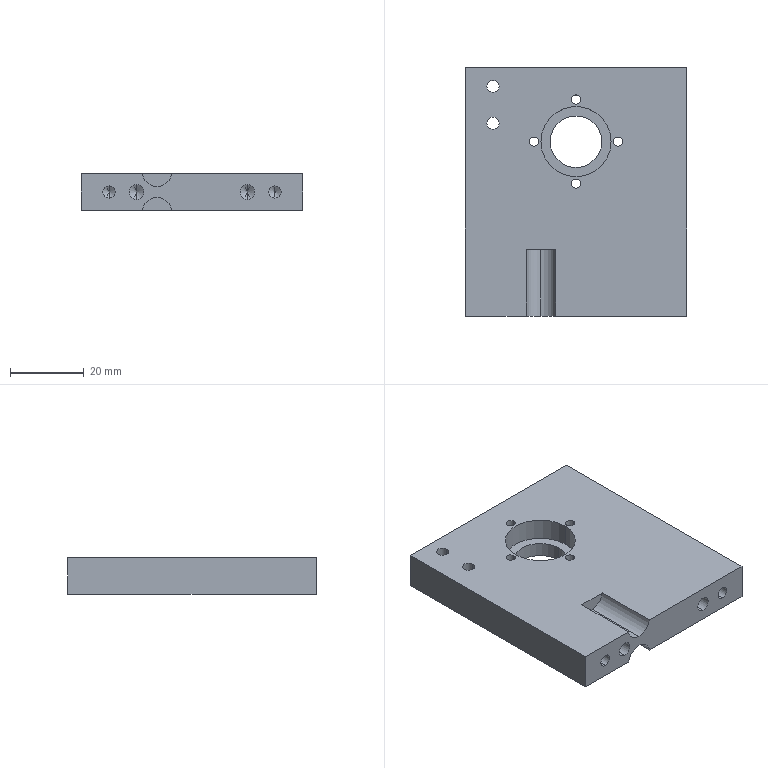Part | STEP file | 11-FG-B00711 | 1 solid | 64 faces | box 60 x 67.3 x 10 mm | volume 36302 mm3 | cylinder 37 | cone 18 | plane 9 | commonest cylinder face diameters 2.5 x18 3.3 x8 4 x4 8 x3 14 x2 19 x2